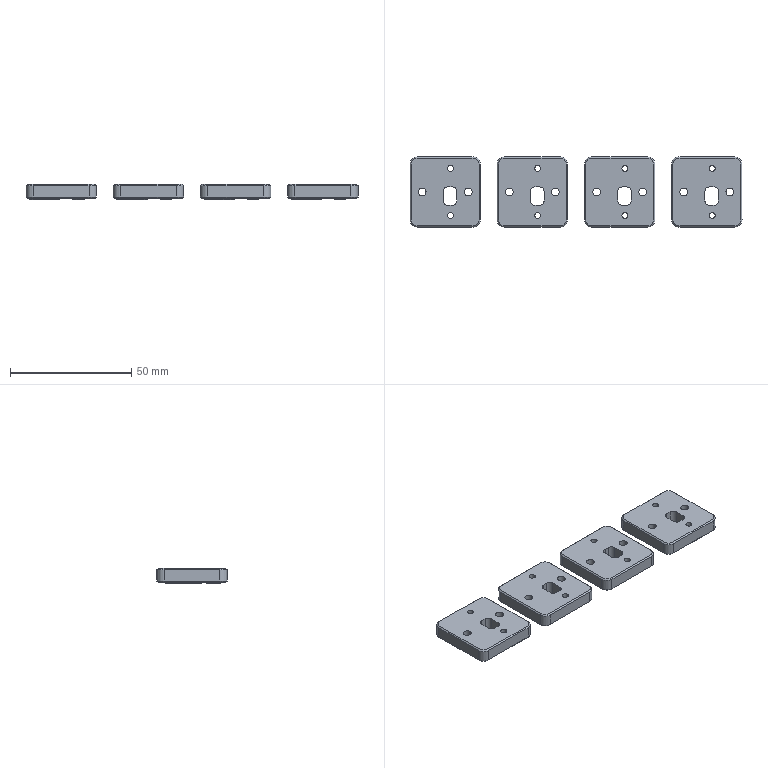Part | 4 solids | 816 faces | box 137 x 29 x 6.3 mm | volume 17628 mm3 | plane 376 | spline 172 | cylinder 148 | cone 120 | commonest cylinder face diameters 1 x56 4 x24 2.5 x16 3.3 x16 3.6 x16 6 x16